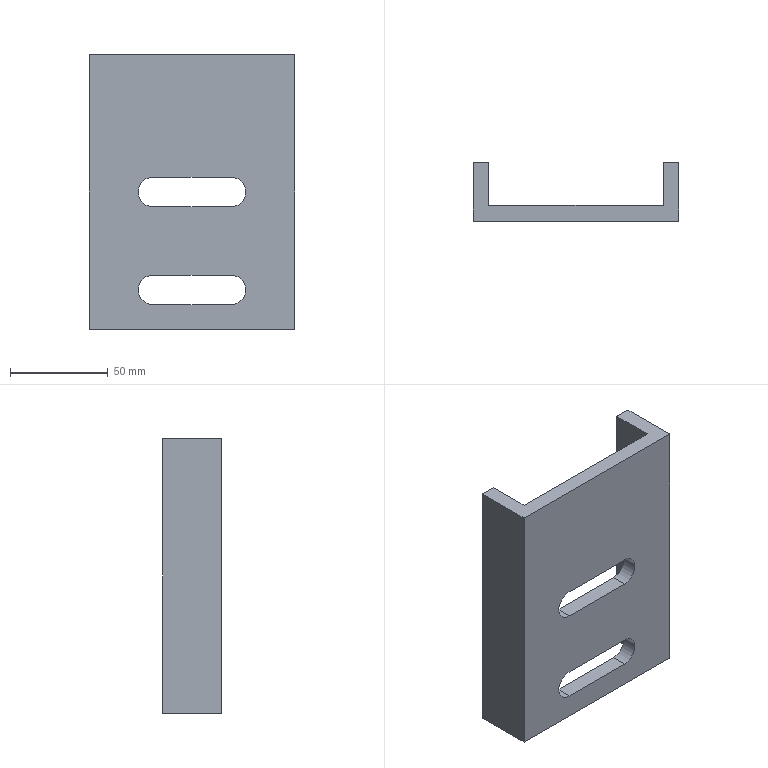Part | SolidWorks | features Extrusion 1, ICE 1 | 1 solid | 18 faces | box 105 x 30 x 140 mm | volume 154453 mm3 | plane 14 | cylinder 4 | commonest cylinder face diameters 15 x4
STEP:
#1=CARTESIAN_POINT('',(0.,0.,0.));
#2=VERTEX_POINT('',#1);
#3=CARTESIAN_POINT('',(105.,0.,0.));
#4=VERTEX_POINT('',#3);
#5=CARTESIAN_POINT('',(0.,0.,0.));
#6=DIRECTION('',(1.,0.,0.));
#7=VECTOR('',#6,1000.);
#8=LINE('',#5,#7);
#9=EDGE_CURVE('',#2,#4,#8,.T.);
#10=ORIENTED_EDGE('',*,*,#9,.T.);
#11=CARTESIAN_POINT('',(105.,0.,140.));
#12=VERTEX_POINT('',#11);
#13=CARTESIAN_POINT('',(105.,0.,140.));
#14=DIRECTION('',(0.,0.,-1.));
#15=VECTOR('',#14,1000.);
#16=LINE('',#13,#15);
#17=EDGE_CURVE('',#12,#4,#16,.T.);
#18=ORIENTED_EDGE('',*,*,#17,.F.);
#19=CARTESIAN_POINT('',(0.,0.,140.));
#20=VERTEX_POINT('',#19);
#21=CARTESIAN_POINT('',(0.,0.,140.));
#22=DIRECTION('',(1.,0.,0.));
#23=VECTOR('',#22,1000.);
#24=LINE('',#21,#23);
#25=EDGE_CURVE('',#20,#12,#24,.T.);
#26=ORIENTED_EDGE('',*,*,#25,.F.);
#27=CARTESIAN_POINT('',(0.,0.,140.));
#28=DIRECTION('',(0.,0.,-1.));
#29=VECTOR('',#28,1000.);
#30=LINE('',#27,#29);
#31=EDGE_CURVE('',#20,#2,#30,.T.);
#32=ORIENTED_EDGE('',*,*,#31,.T.);
#33=EDGE_LOOP('',(#10,#18,#26,#32));
#34=FACE_OUTER_BOUND('',#33,.T.);
#35=CARTESIAN_POINT('',(72.5,0.,62.5));
#36=VERTEX_POINT('',#35);
#37=CARTESIAN_POINT('',(72.5,0.,77.5));
#38=VERTEX_POINT('',#37);
#39=CARTESIAN_POINT('',(72.5,0.,70.));
#40=DIRECTION('',(0.,-1.,0.));
#41=DIRECTION('',(0.,0.,-1.));
#42=AXIS2_PLACEMENT_3D('',#39,#40,#41);
#43=CIRCLE('',#42,7.5);
#44=EDGE_CURVE('',#36,#38,#43,.T.);
#45=ORIENTED_EDGE('',*,*,#44,.F.);
#46=CARTESIAN_POINT('',(32.5,0.,62.5));
#47=VERTEX_POINT('',#46);
#48=CARTESIAN_POINT('',(0.,0.,62.5));
#49=DIRECTION('',(1.,0.,0.));
#50=VECTOR('',#49,1000.);
#51=LINE('',#48,#50);
#52=EDGE_CURVE('',#47,#36,#51,.T.);
#53=ORIENTED_EDGE('',*,*,#52,.F.);
#54=CARTESIAN_POINT('',(32.5,0.,77.5));
#55=VERTEX_POINT('',#54);
#56=CARTESIAN_POINT('',(32.5,0.,70.));
#57=DIRECTION('',(0.,-1.,0.));
#58=DIRECTION('',(0.,0.,-1.));
#59=AXIS2_PLACEMENT_3D('',#56,#57,#58);
#60=CIRCLE('',#59,7.5);
#61=EDGE_CURVE('',#55,#47,#60,.T.);
#62=ORIENTED_EDGE('',*,*,#61,.F.);
#63=CARTESIAN_POINT('',(0.,0.,77.5));
#64=DIRECTION('',(1.,0.,0.));
#65=VECTOR('',#64,1000.);
#66=LINE('',#63,#65);
#67=EDGE_CURVE('',#55,#38,#66,.T.);
#68=ORIENTED_EDGE('',*,*,#67,.T.);
#69=EDGE_LOOP('',(#45,#53,#62,#68));
#70=FACE_BOUND('',#69,.T.);
#71=CARTESIAN_POINT('',(32.5,0.,27.5));
#72=VERTEX_POINT('',#71);
#73=CARTESIAN_POINT('',(72.5,0.,27.5));
#74=VERTEX_POINT('',#73);
#75=CARTESIAN_POINT('',(0.,0.,27.5));
#76=DIRECTION('',(1.,0.,0.));
#77=VECTOR('',#76,1000.);
#78=LINE('',#75,#77);
#79=EDGE_CURVE('',#72,#74,#78,.T.);
#80=ORIENTED_EDGE('',*,*,#79,.T.);
#81=CARTESIAN_POINT('',(72.5,0.,12.5));
#82=VERTEX_POINT('',#81);
#83=CARTESIAN_POINT('',(72.5,0.,20.));
#84=DIRECTION('',(0.,-1.,0.));
#85=DIRECTION('',(0.,0.,-1.));
#86=AXIS2_PLACEMENT_3D('',#83,#84,#85);
#87=CIRCLE('',#86,7.5);
#88=EDGE_CURVE('',#82,#74,#87,.T.);
#89=ORIENTED_EDGE('',*,*,#88,.F.);
#90=CARTESIAN_POINT('',(32.5,0.,12.5));
#91=VERTEX_POINT('',#90);
#92=CARTESIAN_POINT('',(0.,0.,12.5));
#93=DIRECTION('',(1.,0.,0.));
#94=VECTOR('',#93,1000.);
#95=LINE('',#92,#94);
#96=EDGE_CURVE('',#91,#82,#95,.T.);
#97=ORIENTED_EDGE('',*,*,#96,.F.);
#98=CARTESIAN_POINT('',(32.5,0.,20.));
#99=DIRECTION('',(0.,-1.,0.));
#100=DIRECTION('',(0.,0.,-1.));
#101=AXIS2_PLACEMENT_3D('',#98,#99,#100);
#102=CIRCLE('',#101,7.5);
#103=EDGE_CURVE('',#72,#91,#102,.T.);
#104=ORIENTED_EDGE('',*,*,#103,.F.);
#105=EDGE_LOOP('',(#80,#89,#97,#104));
#106=FACE_BOUND('',#105,.T.);
#107=CARTESIAN_POINT('',(0.,0.,140.));
#108=DIRECTION('',(0.,1.,0.));
#109=DIRECTION('',(0.,0.,1.));
#110=AXIS2_PLACEMENT_3D('',#107,#108,#109);
#111=PLANE('',#110);
#112=ADVANCED_FACE('',(#34,#70,#106),#111,.F.);
#113=CARTESIAN_POINT('',(97.,8.,0.));
#114=VERTEX_POINT('',#113);
#115=CARTESIAN_POINT('',(8.,8.,0.));
#116=VERTEX_POINT('',#115);
#117=CARTESIAN_POINT('',(8.,8.,0.));
#118=DIRECTION('',(-1.,0.,0.));
#119=VECTOR('',#118,1000.);
#120=LINE('',#117,#119);
#121=EDGE_CURVE('',#114,#116,#120,.T.);
#122=ORIENTED_EDGE('',*,*,#121,.T.);
#123=CARTESIAN_POINT('',(8.,8.,140.));
#124=VERTEX_POINT('',#123);
#125=CARTESIAN_POINT('',(8.,8.,140.));
#126=DIRECTION('',(0.,0.,-1.));
#127=VECTOR('',#126,1000.);
#128=LINE('',#125,#127);
#129=EDGE_CURVE('',#124,#116,#128,.T.);
#130=ORIENTED_EDGE('',*,*,#129,.F.);
#131=CARTESIAN_POINT('',(97.,8.,140.));
#132=VERTEX_POINT('',#131);
#133=CARTESIAN_POINT('',(8.,8.,140.));
#134=DIRECTION('',(-1.,0.,0.));
#135=VECTOR('',#134,1000.);
#136=LINE('',#133,#135);
#137=EDGE_CURVE('',#132,#124,#136,.T.);
#138=ORIENTED_EDGE('',*,*,#137,.F.);
#139=CARTESIAN_POINT('',(97.,8.,140.));
#140=DIRECTION('',(0.,0.,-1.));
#141=VECTOR('',#140,1000.);
#142=LINE('',#139,#141);
#143=EDGE_CURVE('',#132,#114,#142,.T.);
#144=ORIENTED_EDGE('',*,*,#143,.T.);
#145=EDGE_LOOP('',(#122,#130,#138,#144));
#146=FACE_OUTER_BOUND('',#145,.T.);
#147=CARTESIAN_POINT('',(32.5,8.,77.5));
#148=VERTEX_POINT('',#147);
#149=CARTESIAN_POINT('',(32.5,8.,62.5));
#150=VERTEX_POINT('',#149);
#151=CARTESIAN_POINT('',(32.5,8.,70.));
#152=DIRECTION('',(0.,-1.,0.));
#153=DIRECTION('',(0.,0.,-1.));
#154=AXIS2_PLACEMENT_3D('',#151,#152,#153);
#155=CIRCLE('',#154,7.5);
#156=EDGE_CURVE('',#148,#150,#155,.T.);
#157=ORIENTED_EDGE('',*,*,#156,.T.);
#158=CARTESIAN_POINT('',(72.5,8.,62.5));
#159=VERTEX_POINT('',#158);
#160=CARTESIAN_POINT('',(8.,8.,62.5));
#161=DIRECTION('',(1.,0.,0.));
#162=VECTOR('',#161,1000.);
#163=LINE('',#160,#162);
#164=EDGE_CURVE('',#150,#159,#163,.T.);
#165=ORIENTED_EDGE('',*,*,#164,.T.);
#166=CARTESIAN_POINT('',(72.5,8.,77.5));
#167=VERTEX_POINT('',#166);
#168=CARTESIAN_POINT('',(72.5,8.,70.));
#169=DIRECTION('',(0.,-1.,0.));
#170=DIRECTION('',(0.,0.,-1.));
#171=AXIS2_PLACEMENT_3D('',#168,#169,#170);
#172=CIRCLE('',#171,7.5);
#173=EDGE_CURVE('',#159,#167,#172,.T.);
#174=ORIENTED_EDGE('',*,*,#173,.T.);
#175=CARTESIAN_POINT('',(8.,8.,77.5));
#176=DIRECTION('',(1.,0.,0.));
#177=VECTOR('',#176,1000.);
#178=LINE('',#175,#177);
#179=EDGE_CURVE('',#148,#167,#178,.T.);
#180=ORIENTED_EDGE('',*,*,#179,.F.);
#181=EDGE_LOOP('',(#157,#165,#174,#180));
#182=FACE_BOUND('',#181,.T.);
#183=CARTESIAN_POINT('',(32.5,8.,27.5));
#184=VERTEX_POINT('',#183);
#185=CARTESIAN_POINT('',(72.5,8.,27.5));
#186=VERTEX_POINT('',#185);
#187=CARTESIAN_POINT('',(8.,8.,27.5));
#188=DIRECTION('',(1.,0.,0.));
#189=VECTOR('',#188,1000.);
#190=LINE('',#187,#189);
#191=EDGE_CURVE('',#184,#186,#190,.T.);
#192=ORIENTED_EDGE('',*,*,#191,.F.);
#193=CARTESIAN_POINT('',(32.5,8.,12.5));
#194=VERTEX_POINT('',#193);
#195=CARTESIAN_POINT('',(32.5,8.,20.));
#196=DIRECTION('',(0.,-1.,0.));
#197=DIRECTION('',(0.,0.,-1.));
#198=AXIS2_PLACEMENT_3D('',#195,#196,#197);
#199=CIRCLE('',#198,7.5);
#200=EDGE_CURVE('',#184,#194,#199,.T.);
#201=ORIENTED_EDGE('',*,*,#200,.T.);
#202=CARTESIAN_POINT('',(72.5,8.,12.5));
#203=VERTEX_POINT('',#202);
#204=CARTESIAN_POINT('',(8.,8.,12.5));
#205=DIRECTION('',(1.,0.,0.));
#206=VECTOR('',#205,1000.);
#207=LINE('',#204,#206);
#208=EDGE_CURVE('',#194,#203,#207,.T.);
#209=ORIENTED_EDGE('',*,*,#208,.T.);
#210=CARTESIAN_POINT('',(72.5,8.,20.));
#211=DIRECTION('',(0.,-1.,0.));
#212=DIRECTION('',(0.,0.,-1.));
#213=AXIS2_PLACEMENT_3D('',#210,#211,#212);
#214=CIRCLE('',#213,7.5);
#215=EDGE_CURVE('',#203,#186,#214,.T.);
#216=ORIENTED_EDGE('',*,*,#215,.T.);
#217=EDGE_LOOP('',(#192,#201,#209,#216));
#218=FACE_BOUND('',#217,.T.);
#219=CARTESIAN_POINT('',(8.,8.,140.));
#220=DIRECTION('',(0.,-1.,0.));
#221=DIRECTION('',(0.,0.,-1.));
#222=AXIS2_PLACEMENT_3D('',#219,#220,#221);
#223=PLANE('',#222);
#224=ADVANCED_FACE('',(#146,#182,#218),#223,.F.);
#225=CARTESIAN_POINT('',(0.,30.,0.));
#226=VERTEX_POINT('',#225);
#227=CARTESIAN_POINT('',(0.,0.,0.));
#228=DIRECTION('',(0.,-1.,0.));
#229=VECTOR('',#228,1000.);
#230=LINE('',#227,#229);
#231=EDGE_CURVE('',#226,#2,#230,.T.);
#232=ORIENTED_EDGE('',*,*,#231,.T.);
#233=ORIENTED_EDGE('',*,*,#31,.F.);
#234=CARTESIAN_POINT('',(0.,30.,140.));
#235=VERTEX_POINT('',#234);
#236=CARTESIAN_POINT('',(0.,0.,140.));
#237=DIRECTION('',(0.,-1.,0.));
#238=VECTOR('',#237,1000.);
#239=LINE('',#236,#238);
#240=EDGE_CURVE('',#235,#20,#239,.T.);
#241=ORIENTED_EDGE('',*,*,#240,.F.);
#242=CARTESIAN_POINT('',(0.,30.,140.));
#243=DIRECTION('',(0.,0.,-1.));
#244=VECTOR('',#243,1000.);
#245=LINE('',#242,#244);
#246=EDGE_CURVE('',#235,#226,#245,.T.);
#247=ORIENTED_EDGE('',*,*,#246,.T.);
#248=EDGE_LOOP('',(#232,#233,#241,#247));
#249=FACE_OUTER_BOUND('',#248,.T.);
#250=CARTESIAN_POINT('',(0.,0.,140.));
#251=DIRECTION('',(1.,0.,0.));
#252=DIRECTION('',(0.,0.,-1.));
#253=AXIS2_PLACEMENT_3D('',#250,#251,#252);
#254=PLANE('',#253);
#255=ADVANCED_FACE('',(#249),#254,.F.);
#256=CARTESIAN_POINT('',(105.,30.,0.));
#257=VERTEX_POINT('',#256);
#258=CARTESIAN_POINT('',(105.,0.,0.));
#259=DIRECTION('',(0.,1.,0.));
#260=VECTOR('',#259,1000.);
#261=LINE('',#258,#260);
#262=EDGE_CURVE('',#4,#257,#261,.T.);
#263=ORIENTED_EDGE('',*,*,#262,.T.);
#264=CARTESIAN_POINT('',(105.,30.,140.));
#265=VERTEX_POINT('',#264);
#266=CARTESIAN_POINT('',(105.,30.,140.));
#267=DIRECTION('',(0.,0.,-1.));
#268=VECTOR('',#267,1000.);
#269=LINE('',#266,#268);
#270=EDGE_CURVE('',#265,#257,#269,.T.);
#271=ORIENTED_EDGE('',*,*,#270,.F.);
#272=CARTESIAN_POINT('',(105.,0.,140.));
#273=DIRECTION('',(0.,1.,0.));
#274=VECTOR('',#273,1000.);
#275=LINE('',#272,#274);
#276=EDGE_CURVE('',#12,#265,#275,.T.);
#277=ORIENTED_EDGE('',*,*,#276,.F.);
#278=ORIENTED_EDGE('',*,*,#17,.T.);
#279=EDGE_LOOP('',(#263,#271,#277,#278));
#280=FACE_OUTER_BOUND('',#279,.T.);
#281=CARTESIAN_POINT('',(105.,0.,140.));
#282=DIRECTION('',(-1.,0.,0.));
#283=DIRECTION('',(0.,0.,1.));
#284=AXIS2_PLACEMENT_3D('',#281,#282,#283);
#285=PLANE('',#284);
#286=ADVANCED_FACE('',(#280),#285,.F.);
#287=CARTESIAN_POINT('',(97.,30.,0.));
#288=VERTEX_POINT('',#287);
#289=CARTESIAN_POINT('',(97.,30.,0.));
#290=DIRECTION('',(-1.,0.,0.));
#291=VECTOR('',#290,1000.);
#292=LINE('',#289,#291);
#293=EDGE_CURVE('',#257,#288,#292,.T.);
#294=ORIENTED_EDGE('',*,*,#293,.T.);
#295=CARTESIAN_POINT('',(97.,30.,140.));
#296=VERTEX_POINT('',#295);
#297=CARTESIAN_POINT('',(97.,30.,140.));
#298=DIRECTION('',(0.,0.,-1.));
#299=VECTOR('',#298,1000.);
#300=LINE('',#297,#299);
#301=EDGE_CURVE('',#296,#288,#300,.T.);
#302=ORIENTED_EDGE('',*,*,#301,.F.);
#303=CARTESIAN_POINT('',(97.,30.,140.));
#304=DIRECTION('',(-1.,0.,0.));
#305=VECTOR('',#304,1000.);
#306=LINE('',#303,#305);
#307=EDGE_CURVE('',#265,#296,#306,.T.);
#308=ORIENTED_EDGE('',*,*,#307,.F.);
#309=ORIENTED_EDGE('',*,*,#270,.T.);
#310=EDGE_LOOP('',(#294,#302,#308,#309));
#311=FACE_OUTER_BOUND('',#310,.T.);
#312=CARTESIAN_POINT('',(97.,30.,140.));
#313=DIRECTION('',(0.,-1.,0.));
#314=DIRECTION('',(0.,0.,-1.));
#315=AXIS2_PLACEMENT_3D('',#312,#313,#314);
#316=PLANE('',#315);
#317=ADVANCED_FACE('',(#311),#316,.F.);
#318=CARTESIAN_POINT('',(97.,8.,0.));
#319=DIRECTION('',(0.,-1.,0.));
#320=VECTOR('',#319,1000.);
#321=LINE('',#318,#320);
#322=EDGE_CURVE('',#288,#114,#321,.T.);
#323=ORIENTED_EDGE('',*,*,#322,.T.);
#324=ORIENTED_EDGE('',*,*,#143,.F.);
#325=CARTESIAN_POINT('',(97.,8.,140.));
#326=DIRECTION('',(0.,-1.,0.));
#327=VECTOR('',#326,1000.);
#328=LINE('',#325,#327);
#329=EDGE_CURVE('',#296,#132,#328,.T.);
#330=ORIENTED_EDGE('',*,*,#329,.F.);
#331=ORIENTED_EDGE('',*,*,#301,.T.);
#332=EDGE_LOOP('',(#323,#324,#330,#331));
#333=FACE_OUTER_BOUND('',#332,.T.);
#334=CARTESIAN_POINT('',(97.,8.,140.));
#335=DIRECTION('',(1.,0.,0.));
#336=DIRECTION('',(0.,0.,-1.));
#337=AXIS2_PLACEMENT_3D('',#334,#335,#336);
#338=PLANE('',#337);
#339=ADVANCED_FACE('',(#333),#338,.F.);
#340=CARTESIAN_POINT('',(8.,30.,0.));
#341=VERTEX_POINT('',#340);
#342=CARTESIAN_POINT('',(8.,8.,0.));
#343=DIRECTION('',(0.,1.,0.));
#344=VECTOR('',#343,1000.);
#345=LINE('',#342,#344);
#346=EDGE_CURVE('',#116,#341,#345,.T.);
#347=ORIENTED_EDGE('',*,*,#346,.T.);
#348=CARTESIAN_POINT('',(8.,30.,140.));
#349=VERTEX_POINT('',#348);
#350=CARTESIAN_POINT('',(8.,30.,140.));
#351=DIRECTION('',(0.,0.,-1.));
#352=VECTOR('',#351,1000.);
#353=LINE('',#350,#352);
#354=EDGE_CURVE('',#349,#341,#353,.T.);
#355=ORIENTED_EDGE('',*,*,#354,.F.);
#356=CARTESIAN_POINT('',(8.,8.,140.));
#357=DIRECTION('',(0.,1.,0.));
#358=VECTOR('',#357,1000.);
#359=LINE('',#356,#358);
#360=EDGE_CURVE('',#124,#349,#359,.T.);
#361=ORIENTED_EDGE('',*,*,#360,.F.);
#362=ORIENTED_EDGE('',*,*,#129,.T.);
#363=EDGE_LOOP('',(#347,#355,#361,#362));
#364=FACE_OUTER_BOUND('',#363,.T.);
#365=CARTESIAN_POINT('',(8.,8.,140.));
#366=DIRECTION('',(-1.,0.,0.));
#367=DIRECTION('',(0.,0.,1.));
#368=AXIS2_PLACEMENT_3D('',#365,#366,#367);
#369=PLANE('',#368);
#370=ADVANCED_FACE('',(#364),#369,.F.);
#371=CARTESIAN_POINT('',(0.,30.,0.));
#372=DIRECTION('',(-1.,0.,0.));
#373=VECTOR('',#372,1000.);
#374=LINE('',#371,#373);
#375=EDGE_CURVE('',#341,#226,#374,.T.);
#376=ORIENTED_EDGE('',*,*,#375,.T.);
#377=ORIENTED_EDGE('',*,*,#246,.F.);
#378=CARTESIAN_POINT('',(0.,30.,140.));
#379=DIRECTION('',(-1.,0.,0.));
#380=VECTOR('',#379,1000.);
#381=LINE('',#378,#380);
#382=EDGE_CURVE('',#349,#235,#381,.T.);
#383=ORIENTED_EDGE('',*,*,#382,.F.);
#384=ORIENTED_EDGE('',*,*,#354,.T.);
#385=EDGE_LOOP('',(#376,#377,#383,#384));
#386=FACE_OUTER_BOUND('',#385,.T.);
#387=CARTESIAN_POINT('',(0.,30.,140.));
#388=DIRECTION('',(0.,-1.,0.));
#389=DIRECTION('',(0.,0.,-1.));
#390=AXIS2_PLACEMENT_3D('',#387,#388,#389);
#391=PLANE('',#390);
#392=ADVANCED_FACE('',(#386),#391,.F.);
#393=ORIENTED_EDGE('',*,*,#240,.T.);
#394=ORIENTED_EDGE('',*,*,#25,.T.);
#395=ORIENTED_EDGE('',*,*,#276,.T.);
#396=ORIENTED_EDGE('',*,*,#307,.T.);
#397=ORIENTED_EDGE('',*,*,#329,.T.);
#398=ORIENTED_EDGE('',*,*,#137,.T.);
#399=ORIENTED_EDGE('',*,*,#360,.T.);
#400=ORIENTED_EDGE('',*,*,#382,.T.);
#401=EDGE_LOOP('',(#393,#394,#395,#396,#397,#398,#399,#400));
#402=FACE_OUTER_BOUND('',#401,.T.);
#403=CARTESIAN_POINT('',(0.,0.,140.));
#404=DIRECTION('',(0.,0.,-1.));
#405=DIRECTION('',(-1.,0.,0.));
#406=AXIS2_PLACEMENT_3D('',#403,#404,#405);
#407=PLANE('',#406);
#408=ADVANCED_FACE('',(#402),#407,.F.);
#409=ORIENTED_EDGE('',*,*,#231,.F.);
#410=ORIENTED_EDGE('',*,*,#375,.F.);
#411=ORIENTED_EDGE('',*,*,#346,.F.);
#412=ORIENTED_EDGE('',*,*,#121,.F.);
#413=ORIENTED_EDGE('',*,*,#322,.F.);
#414=ORIENTED_EDGE('',*,*,#293,.F.);
#415=ORIENTED_EDGE('',*,*,#262,.F.);
#416=ORIENTED_EDGE('',*,*,#9,.F.);
#417=EDGE_LOOP('',(#409,#410,#411,#412,#413,#414,#415,#416));
#418=FACE_OUTER_BOUND('',#417,.T.);
#419=CARTESIAN_POINT('',(0.,0.,0.));
#420=DIRECTION('',(0.,0.,-1.));
#421=DIRECTION('',(-1.,0.,0.));
#422=AXIS2_PLACEMENT_3D('',#419,#420,#421);
#423=PLANE('',#422);
#424=ADVANCED_FACE('',(#418),#423,.T.);
#425=CARTESIAN_POINT('',(32.5,140.,62.5));
#426=DIRECTION('',(0.,-1.,0.));
#427=VECTOR('',#426,1000.);
#428=LINE('',#425,#427);
#429=EDGE_CURVE('',#150,#47,#428,.T.);
#430=ORIENTED_EDGE('',*,*,#429,.T.);
#431=ORIENTED_EDGE('',*,*,#52,.T.);
#432=CARTESIAN_POINT('',(72.5,140.,62.5));
#433=DIRECTION('',(0.,-1.,0.));
#434=VECTOR('',#433,1000.);
#435=LINE('',#432,#434);
#436=EDGE_CURVE('',#159,#36,#435,.T.);
#437=ORIENTED_EDGE('',*,*,#436,.F.);
#438=ORIENTED_EDGE('',*,*,#164,.F.);
#439=EDGE_LOOP('',(#430,#431,#437,#438));
#440=FACE_OUTER_BOUND('',#439,.T.);
#441=CARTESIAN_POINT('',(0.,140.,62.5));
#442=DIRECTION('',(0.,0.,-1.));
#443=DIRECTION('',(-1.,0.,0.));
#444=AXIS2_PLACEMENT_3D('',#441,#442,#443);
#445=PLANE('',#444);
#446=ADVANCED_FACE('',(#440),#445,.F.);
#447=CARTESIAN_POINT('',(32.5,140.,77.5));
#448=DIRECTION('',(0.,-1.,0.));
#449=VECTOR('',#448,1000.);
#450=LINE('',#447,#449);
#451=EDGE_CURVE('',#148,#55,#450,.T.);
#452=ORIENTED_EDGE('',*,*,#451,.T.);
#453=ORIENTED_EDGE('',*,*,#61,.T.);
#454=ORIENTED_EDGE('',*,*,#429,.F.);
#455=ORIENTED_EDGE('',*,*,#156,.F.);
#456=EDGE_LOOP('',(#452,#453,#454,#455));
#457=FACE_OUTER_BOUND('',#456,.T.);
#458=CARTESIAN_POINT('',(32.5,140.,70.));
#459=DIRECTION('',(0.,-1.,0.));
#460=DIRECTION('',(0.,0.,-1.));
#461=AXIS2_PLACEMENT_3D('',#458,#459,#460);
#462=CYLINDRICAL_SURFACE('',#461,7.5);
#463=ADVANCED_FACE('',(#457),#462,.F.);
#464=ORIENTED_EDGE('',*,*,#179,.T.);
#465=CARTESIAN_POINT('',(72.5,140.,77.5));
#466=DIRECTION('',(0.,-1.,0.));
#467=VECTOR('',#466,1000.);
#468=LINE('',#465,#467);
#469=EDGE_CURVE('',#167,#38,#468,.T.);
#470=ORIENTED_EDGE('',*,*,#469,.T.);
#471=ORIENTED_EDGE('',*,*,#67,.F.);
#472=ORIENTED_EDGE('',*,*,#451,.F.);
#473=EDGE_LOOP('',(#464,#470,#471,#472));
#474=FACE_OUTER_BOUND('',#473,.T.);
#475=CARTESIAN_POINT('',(0.,140.,77.5));
#476=DIRECTION('',(0.,0.,-1.));
#477=DIRECTION('',(-1.,0.,0.));
#478=AXIS2_PLACEMENT_3D('',#475,#476,#477);
#479=PLANE('',#478);
#480=ADVANCED_FACE('',(#474),#479,.T.);
#481=ORIENTED_EDGE('',*,*,#436,.T.);
#482=ORIENTED_EDGE('',*,*,#44,.T.);
#483=ORIENTED_EDGE('',*,*,#469,.F.);
#484=ORIENTED_EDGE('',*,*,#173,.F.);
#485=EDGE_LOOP('',(#481,#482,#483,#484));
#486=FACE_OUTER_BOUND('',#485,.T.);
#487=CARTESIAN_POINT('',(72.5,140.,70.));
#488=DIRECTION('',(0.,-1.,0.));
#489=DIRECTION('',(0.,0.,-1.));
#490=AXIS2_PLACEMENT_3D('',#487,#488,#489);
#491=CYLINDRICAL_SURFACE('',#490,7.5);
#492=ADVANCED_FACE('',(#486),#491,.F.);
#493=ORIENTED_EDGE('',*,*,#191,.T.);
#494=CARTESIAN_POINT('',(72.5,140.,27.5));
#495=DIRECTION('',(0.,-1.,0.));
#496=VECTOR('',#495,1000.);
#497=LINE('',#494,#496);
#498=EDGE_CURVE('',#186,#74,#497,.T.);
#499=ORIENTED_EDGE('',*,*,#498,.T.);
#500=ORIENTED_EDGE('',*,*,#79,.F.);
#501=CARTESIAN_POINT('',(32.5,140.,27.5));
#502=DIRECTION('',(0.,-1.,0.));
#503=VECTOR('',#502,1000.);
#504=LINE('',#501,#503);
#505=EDGE_CURVE('',#184,#72,#504,.T.);
#506=ORIENTED_EDGE('',*,*,#505,.F.);
#507=EDGE_LOOP('',(#493,#499,#500,#506));
#508=FACE_OUTER_BOUND('',#507,.T.);
#509=CARTESIAN_POINT('',(0.,140.,27.5));
#510=DIRECTION('',(0.,0.,-1.));
#511=DIRECTION('',(-1.,0.,0.));
#512=AXIS2_PLACEMENT_3D('',#509,#510,#511);
#513=PLANE('',#512);
#514=ADVANCED_FACE('',(#508),#513,.T.);
#515=CARTESIAN_POINT('',(72.5,140.,12.5));
#516=DIRECTION('',(0.,-1.,0.));
#517=VECTOR('',#516,1000.);
#518=LINE('',#515,#517);
#519=EDGE_CURVE('',#203,#82,#518,.T.);
#520=ORIENTED_EDGE('',*,*,#519,.T.);
#521=ORIENTED_EDGE('',*,*,#88,.T.);
#522=ORIENTED_EDGE('',*,*,#498,.F.);
#523=ORIENTED_EDGE('',*,*,#215,.F.);
#524=EDGE_LOOP('',(#520,#521,#522,#523));
#525=FACE_OUTER_BOUND('',#524,.T.);
#526=CARTESIAN_POINT('',(72.5,140.,20.));
#527=DIRECTION('',(0.,-1.,0.));
#528=DIRECTION('',(0.,0.,-1.));
#529=AXIS2_PLACEMENT_3D('',#526,#527,#528);
#530=CYLINDRICAL_SURFACE('',#529,7.5);
#531=ADVANCED_FACE('',(#525),#530,.F.);
#532=CARTESIAN_POINT('',(32.5,140.,12.5));
#533=DIRECTION('',(0.,-1.,0.));
#534=VECTOR('',#533,1000.);
#535=LINE('',#532,#534);
#536=EDGE_CURVE('',#194,#91,#535,.T.);
#537=ORIENTED_EDGE('',*,*,#536,.T.);
#538=ORIENTED_EDGE('',*,*,#96,.T.);
#539=ORIENTED_EDGE('',*,*,#519,.F.);
#540=ORIENTED_EDGE('',*,*,#208,.F.);
#541=EDGE_LOOP('',(#537,#538,#539,#540));
#542=FACE_OUTER_BOUND('',#541,.T.);
#543=CARTESIAN_POINT('',(0.,140.,12.5));
#544=DIRECTION('',(0.,0.,-1.));
#545=DIRECTION('',(-1.,0.,0.));
#546=AXIS2_PLACEMENT_3D('',#543,#544,#545);
#547=PLANE('',#546);
#548=ADVANCED_FACE('',(#542),#547,.F.);
#549=ORIENTED_EDGE('',*,*,#505,.T.);
#550=ORIENTED_EDGE('',*,*,#103,.T.);
#551=ORIENTED_EDGE('',*,*,#536,.F.);
#552=ORIENTED_EDGE('',*,*,#200,.F.);
#553=EDGE_LOOP('',(#549,#550,#551,#552));
#554=FACE_OUTER_BOUND('',#553,.T.);
#555=CARTESIAN_POINT('',(32.5,140.,20.));
#556=DIRECTION('',(0.,-1.,0.));
#557=DIRECTION('',(0.,0.,-1.));
#558=AXIS2_PLACEMENT_3D('',#555,#556,#557);
#559=CYLINDRICAL_SURFACE('',#558,7.5);
#560=ADVANCED_FACE('',(#554),#559,.F.);
#561=CLOSED_SHELL('',(#112,#224,#255,#286,#317,#339,#370,#392,#408,#424,#446,#463,#480,#492,#514,#531,#548,#560));
#562=MANIFOLD_SOLID_BREP('',#561);
#563=CARTESIAN_POINT('',(0.,0.,0.));
#564=DIRECTION('',(0.,0.,1.));
#565=DIRECTION('',(1.,0.,0.));
#566=AXIS2_PLACEMENT_3D('',#563,#564,#565);
#567=(LENGTH_UNIT()NAMED_UNIT(*)SI_UNIT(.MILLI.,.METRE.));
#568=UNCERTAINTY_MEASURE_WITH_UNIT(LENGTH_MEASURE(0.00001),#567,'','');
#569=(NAMED_UNIT(*)PLANE_ANGLE_UNIT()SI_UNIT($,.RADIAN.));
#570=(NAMED_UNIT(*)SI_UNIT($,.STERADIAN.)SOLID_ANGLE_UNIT());
#571=(GEOMETRIC_REPRESENTATION_CONTEXT(3)GLOBAL_UNCERTAINTY_ASSIGNED_CONTEXT((#568))GLOBAL_UNIT_ASSIGNED_CONTEXT((#567,#569,#570))REPRESENTATION_CONTEXT('',''));
#572=ADVANCED_BREP_SHAPE_REPRESENTATION('',(#562,#566),#571);